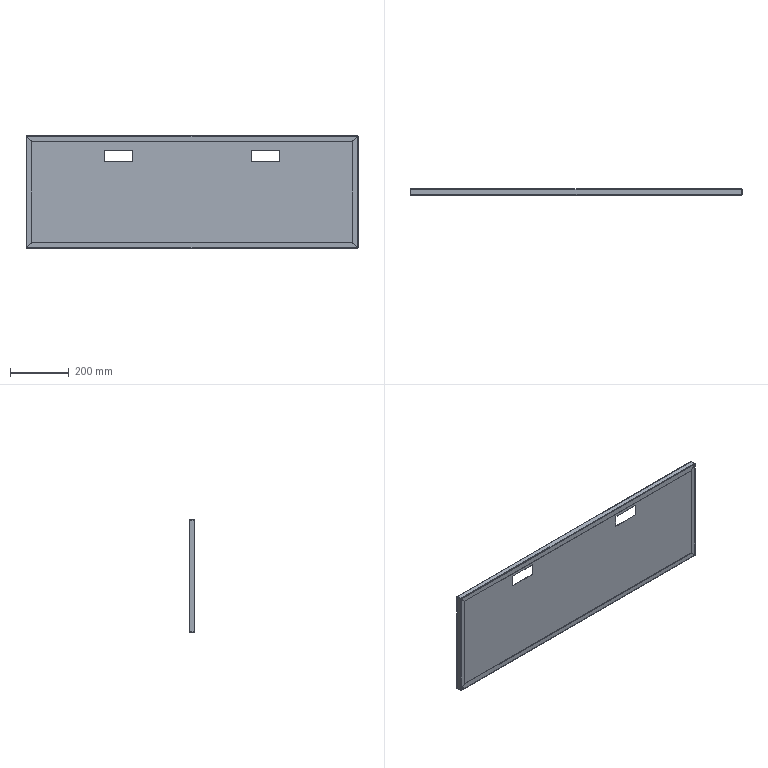Part | SolidWorks | features EdgeFlange 2, FlatPattern 1, ICE 1, SMBaseFlange 1, SheetMetal 1 | 1 solid | 78 faces | box 1135 x 20 x 386 mm | volume 646370 mm3 | plane 46 | spline 16 | cylinder 16 | commonest cylinder face diameters 2 x8 4.4 x8